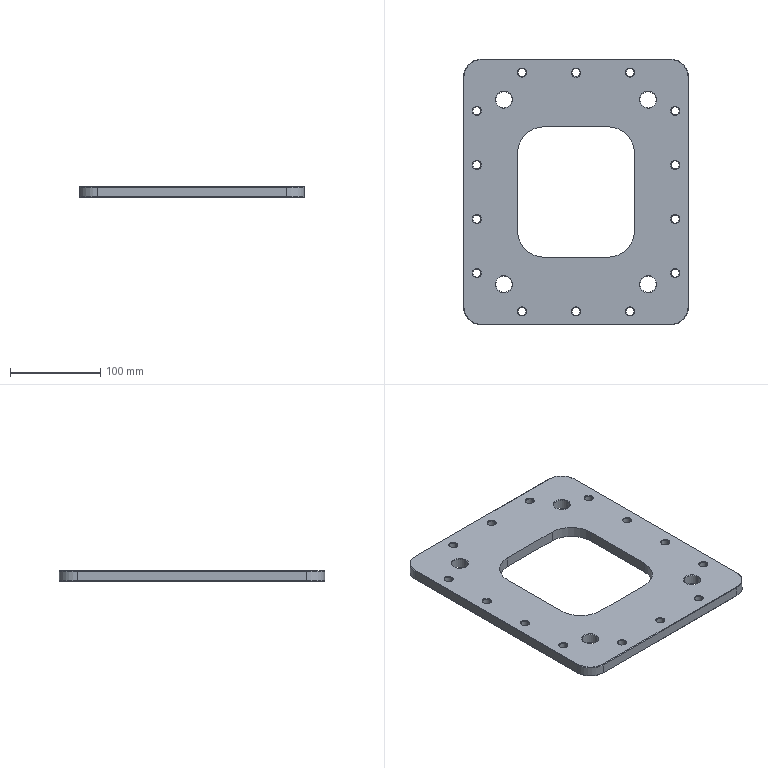Part | SolidWorks | features BaseBody 1 | 1 solid | 142 faces | box 250 x 295 x 12 mm | volume 640437 mm3 | cone 80 | cylinder 44 | plane 18 | commonest cylinder face diameters 9 x28 18 x8 40 x4 60 x4